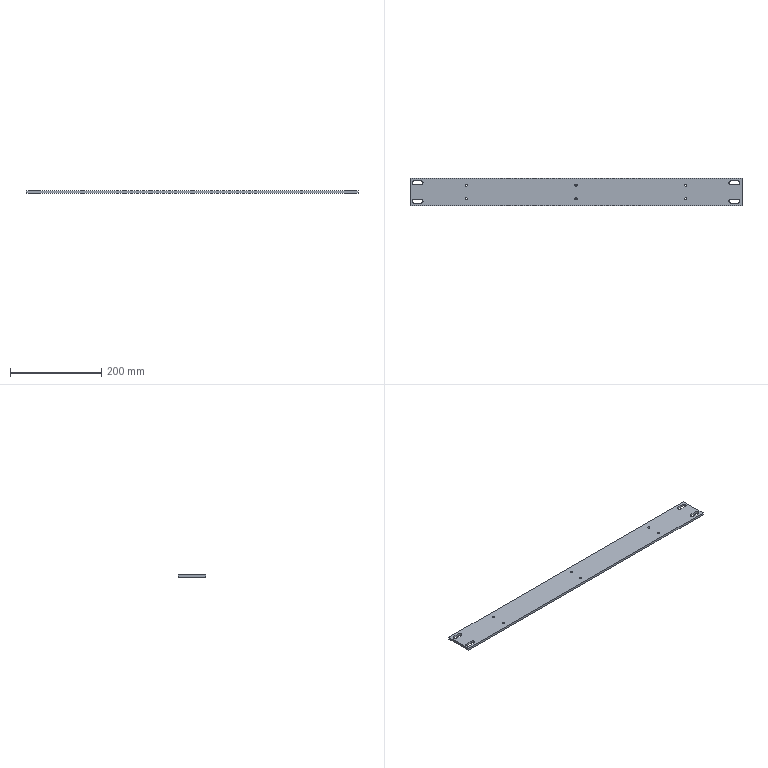Part | STEP file | 1 solid | 38 faces | box 726 x 60 x 5 mm | volume 213239 mm3 | cylinder 24 | plane 14 | commonest cylinder face diameters 5 x12 9 x12